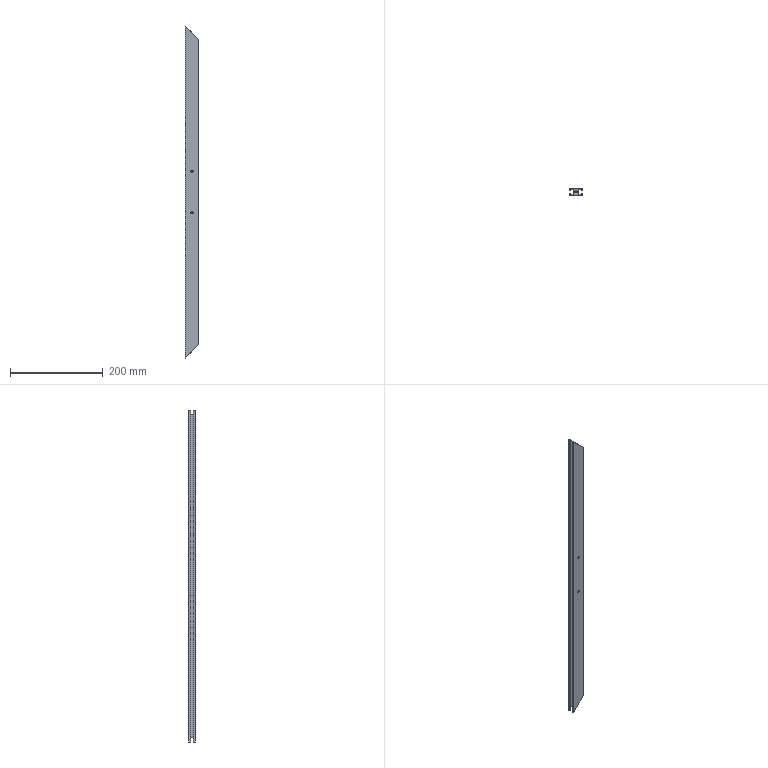Part | SolidWorks | features Extrusion 1, HoleWzd 1, ICE 1 | 1 solid | 37 faces | box 30 x 15 x 717 mm | volume 163444 mm3 | plane 20 | cylinder 17 | commonest cylinder face diameters 5 x14 16.345 x2 16.33 x1
STEP:
#1=CARTESIAN_POINT('',(2375.427,422.907,-45.));
#2=VERTEX_POINT('',#1);
#3=CARTESIAN_POINT('',(2377.927,425.407,-47.5));
#4=VERTEX_POINT('',#3);
#5=CARTESIAN_POINT('',(2375.427,422.907,-45.));
#6=CARTESIAN_POINT('',(2375.427,424.371,-46.464));
#7=CARTESIAN_POINT('',(2376.463,425.407,-47.5));
#8=CARTESIAN_POINT('',(2377.927,425.407,-47.5));
#9=(BOUNDED_CURVE()B_SPLINE_CURVE(3,(#5,#6,#7,#8),.UNSPECIFIED.,.F.,.F.)B_SPLINE_CURVE_WITH_KNOTS((4,4),(4.712,6.283),.UNSPECIFIED.)CURVE()GEOMETRIC_REPRESENTATION_ITEM()RATIONAL_B_SPLINE_CURVE((1.,0.8047,0.8047,1.))REPRESENTATION_ITEM(''));
#10=EDGE_CURVE('',#2,#4,#9,.T.);
#11=ORIENTED_EDGE('',*,*,#10,.T.);
#12=CARTESIAN_POINT('',(2377.927,430.407,-47.5));
#13=VERTEX_POINT('',#12);
#14=CARTESIAN_POINT('',(2377.927,430.407,-47.5));
#15=DIRECTION('',(0.,1.,0.));
#16=VECTOR('',#15,1000.);
#17=LINE('',#14,#16);
#18=EDGE_CURVE('',#4,#13,#17,.T.);
#19=ORIENTED_EDGE('',*,*,#18,.T.);
#20=CARTESIAN_POINT('',(2377.927,430.407,-42.5));
#21=VERTEX_POINT('',#20);
#22=CARTESIAN_POINT('',(2377.927,430.407,-45.));
#23=DIRECTION('',(0.,1.,0.));
#24=DIRECTION('',(0.,0.,1.));
#25=AXIS2_PLACEMENT_3D('',#22,#23,#24);
#26=CIRCLE('',#25,2.5);
#27=EDGE_CURVE('',#13,#21,#26,.T.);
#28=ORIENTED_EDGE('',*,*,#27,.T.);
#29=CARTESIAN_POINT('',(2377.927,425.407,-42.5));
#30=VERTEX_POINT('',#29);
#31=CARTESIAN_POINT('',(2377.927,430.407,-42.5));
#32=DIRECTION('',(0.,1.,0.));
#33=VECTOR('',#32,1000.);
#34=LINE('',#31,#33);
#35=EDGE_CURVE('',#30,#21,#34,.T.);
#36=ORIENTED_EDGE('',*,*,#35,.F.);
#37=CARTESIAN_POINT('',(2377.927,425.407,-42.5));
#38=CARTESIAN_POINT('',(2376.463,425.407,-42.5));
#39=CARTESIAN_POINT('',(2375.427,424.371,-43.536));
#40=CARTESIAN_POINT('',(2375.427,422.907,-45.));
#41=(BOUNDED_CURVE()B_SPLINE_CURVE(3,(#37,#38,#39,#40),.UNSPECIFIED.,.F.,.F.)B_SPLINE_CURVE_WITH_KNOTS((4,4),(3.142,4.712),.UNSPECIFIED.)CURVE()GEOMETRIC_REPRESENTATION_ITEM()RATIONAL_B_SPLINE_CURVE((1.,0.8047,0.8047,1.))REPRESENTATION_ITEM(''));
#42=EDGE_CURVE('',#30,#2,#41,.T.);
#43=ORIENTED_EDGE('',*,*,#42,.T.);
#44=EDGE_LOOP('',(#11,#19,#28,#36,#43));
#45=FACE_OUTER_BOUND('',#44,.T.);
#46=CARTESIAN_POINT('',(2377.927,430.407,-45.));
#47=DIRECTION('',(0.,1.,0.));
#48=DIRECTION('',(0.,0.,1.));
#49=AXIS2_PLACEMENT_3D('',#46,#47,#48);
#50=CYLINDRICAL_SURFACE('',#49,2.5);
#51=ADVANCED_FACE('',(#45),#50,.F.);
#52=CARTESIAN_POINT('',(2377.927,415.407,-47.5));
#53=VERTEX_POINT('',#52);
#54=CARTESIAN_POINT('',(2377.927,415.407,-42.5));
#55=VERTEX_POINT('',#54);
#56=CARTESIAN_POINT('',(2377.927,415.407,-45.));
#57=DIRECTION('',(0.,1.,0.));
#58=DIRECTION('',(0.,0.,1.));
#59=AXIS2_PLACEMENT_3D('',#56,#57,#58);
#60=CIRCLE('',#59,2.5);
#61=EDGE_CURVE('',#53,#55,#60,.T.);
#62=ORIENTED_EDGE('',*,*,#61,.F.);
#63=CARTESIAN_POINT('',(2377.927,420.407,-47.5));
#64=VERTEX_POINT('',#63);
#65=CARTESIAN_POINT('',(2377.927,430.407,-47.5));
#66=DIRECTION('',(0.,1.,0.));
#67=VECTOR('',#66,1000.);
#68=LINE('',#65,#67);
#69=EDGE_CURVE('',#53,#64,#68,.T.);
#70=ORIENTED_EDGE('',*,*,#69,.T.);
#71=CARTESIAN_POINT('',(2377.927,420.407,-47.5));
#72=CARTESIAN_POINT('',(2376.463,420.407,-47.5));
#73=CARTESIAN_POINT('',(2375.427,421.442,-46.464));
#74=CARTESIAN_POINT('',(2375.427,422.907,-45.));
#75=(BOUNDED_CURVE()B_SPLINE_CURVE(3,(#71,#72,#73,#74),.UNSPECIFIED.,.F.,.F.)B_SPLINE_CURVE_WITH_KNOTS((4,4),(0.,1.571),.UNSPECIFIED.)CURVE()GEOMETRIC_REPRESENTATION_ITEM()RATIONAL_B_SPLINE_CURVE((1.,0.8047,0.8047,1.))REPRESENTATION_ITEM(''));
#76=EDGE_CURVE('',#64,#2,#75,.T.);
#77=ORIENTED_EDGE('',*,*,#76,.T.);
#78=CARTESIAN_POINT('',(2377.927,420.407,-42.5));
#79=VERTEX_POINT('',#78);
#80=CARTESIAN_POINT('',(2375.427,422.907,-45.));
#81=CARTESIAN_POINT('',(2375.427,421.442,-43.536));
#82=CARTESIAN_POINT('',(2376.463,420.407,-42.5));
#83=CARTESIAN_POINT('',(2377.927,420.407,-42.5));
#84=(BOUNDED_CURVE()B_SPLINE_CURVE(3,(#80,#81,#82,#83),.UNSPECIFIED.,.F.,.F.)B_SPLINE_CURVE_WITH_KNOTS((4,4),(1.571,3.142),.UNSPECIFIED.)CURVE()GEOMETRIC_REPRESENTATION_ITEM()RATIONAL_B_SPLINE_CURVE((1.,0.8047,0.8047,1.))REPRESENTATION_ITEM(''));
#85=EDGE_CURVE('',#2,#79,#84,.T.);
#86=ORIENTED_EDGE('',*,*,#85,.T.);
#87=CARTESIAN_POINT('',(2377.927,430.407,-42.5));
#88=DIRECTION('',(0.,1.,0.));
#89=VECTOR('',#88,1000.);
#90=LINE('',#87,#89);
#91=EDGE_CURVE('',#55,#79,#90,.T.);
#92=ORIENTED_EDGE('',*,*,#91,.F.);
#93=EDGE_LOOP('',(#62,#70,#77,#86,#92));
#94=FACE_OUTER_BOUND('',#93,.T.);
#95=CARTESIAN_POINT('',(2377.927,430.407,-45.));
#96=DIRECTION('',(0.,1.,0.));
#97=DIRECTION('',(0.,0.,1.));
#98=AXIS2_PLACEMENT_3D('',#95,#96,#97);
#99=CYLINDRICAL_SURFACE('',#98,2.5);
#100=ADVANCED_FACE('',(#94),#99,.F.);
#101=CARTESIAN_POINT('',(2375.427,422.907,45.));
#102=VERTEX_POINT('',#101);
#103=CARTESIAN_POINT('',(2377.927,425.407,42.5));
#104=VERTEX_POINT('',#103);
#105=CARTESIAN_POINT('',(2375.427,422.907,45.));
#106=CARTESIAN_POINT('',(2375.427,424.371,43.536));
#107=CARTESIAN_POINT('',(2376.463,425.407,42.5));
#108=CARTESIAN_POINT('',(2377.927,425.407,42.5));
#109=(BOUNDED_CURVE()B_SPLINE_CURVE(3,(#105,#106,#107,#108),.UNSPECIFIED.,.F.,.F.)B_SPLINE_CURVE_WITH_KNOTS((4,4),(4.712,6.283),.UNSPECIFIED.)CURVE()GEOMETRIC_REPRESENTATION_ITEM()RATIONAL_B_SPLINE_CURVE((1.,0.8047,0.8047,1.))REPRESENTATION_ITEM(''));
#110=EDGE_CURVE('',#102,#104,#109,.T.);
#111=ORIENTED_EDGE('',*,*,#110,.T.);
#112=CARTESIAN_POINT('',(2377.927,430.407,42.5));
#113=VERTEX_POINT('',#112);
#114=CARTESIAN_POINT('',(2377.927,430.407,42.5));
#115=DIRECTION('',(0.,1.,0.));
#116=VECTOR('',#115,1000.);
#117=LINE('',#114,#116);
#118=EDGE_CURVE('',#104,#113,#117,.T.);
#119=ORIENTED_EDGE('',*,*,#118,.T.);
#120=CARTESIAN_POINT('',(2377.927,430.407,47.5));
#121=VERTEX_POINT('',#120);
#122=CARTESIAN_POINT('',(2377.927,430.407,45.));
#123=DIRECTION('',(0.,1.,0.));
#124=DIRECTION('',(0.,0.,1.));
#125=AXIS2_PLACEMENT_3D('',#122,#123,#124);
#126=CIRCLE('',#125,2.5);
#127=EDGE_CURVE('',#113,#121,#126,.T.);
#128=ORIENTED_EDGE('',*,*,#127,.T.);
#129=CARTESIAN_POINT('',(2377.927,425.407,47.5));
#130=VERTEX_POINT('',#129);
#131=CARTESIAN_POINT('',(2377.927,430.407,47.5));
#132=DIRECTION('',(0.,1.,0.));
#133=VECTOR('',#132,1000.);
#134=LINE('',#131,#133);
#135=EDGE_CURVE('',#130,#121,#134,.T.);
#136=ORIENTED_EDGE('',*,*,#135,.F.);
#137=CARTESIAN_POINT('',(2377.927,425.407,47.5));
#138=CARTESIAN_POINT('',(2376.463,425.407,47.5));
#139=CARTESIAN_POINT('',(2375.427,424.371,46.464));
#140=CARTESIAN_POINT('',(2375.427,422.907,45.));
#141=(BOUNDED_CURVE()B_SPLINE_CURVE(3,(#137,#138,#139,#140),.UNSPECIFIED.,.F.,.F.)B_SPLINE_CURVE_WITH_KNOTS((4,4),(3.142,4.712),.UNSPECIFIED.)CURVE()GEOMETRIC_REPRESENTATION_ITEM()RATIONAL_B_SPLINE_CURVE((1.,0.8047,0.8047,1.))REPRESENTATION_ITEM(''));
#142=EDGE_CURVE('',#130,#102,#141,.T.);
#143=ORIENTED_EDGE('',*,*,#142,.T.);
#144=EDGE_LOOP('',(#111,#119,#128,#136,#143));
#145=FACE_OUTER_BOUND('',#144,.T.);
#146=CARTESIAN_POINT('',(2377.927,430.407,45.));
#147=DIRECTION('',(0.,1.,0.));
#148=DIRECTION('',(0.,0.,1.));
#149=AXIS2_PLACEMENT_3D('',#146,#147,#148);
#150=CYLINDRICAL_SURFACE('',#149,2.5);
#151=ADVANCED_FACE('',(#145),#150,.F.);
#152=CARTESIAN_POINT('',(2377.927,415.407,42.5));
#153=VERTEX_POINT('',#152);
#154=CARTESIAN_POINT('',(2377.927,415.407,47.5));
#155=VERTEX_POINT('',#154);
#156=CARTESIAN_POINT('',(2377.927,415.407,45.));
#157=DIRECTION('',(0.,1.,0.));
#158=DIRECTION('',(0.,0.,1.));
#159=AXIS2_PLACEMENT_3D('',#156,#157,#158);
#160=CIRCLE('',#159,2.5);
#161=EDGE_CURVE('',#153,#155,#160,.T.);
#162=ORIENTED_EDGE('',*,*,#161,.F.);
#163=CARTESIAN_POINT('',(2377.927,420.407,42.5));
#164=VERTEX_POINT('',#163);
#165=CARTESIAN_POINT('',(2377.927,430.407,42.5));
#166=DIRECTION('',(0.,1.,0.));
#167=VECTOR('',#166,1000.);
#168=LINE('',#165,#167);
#169=EDGE_CURVE('',#153,#164,#168,.T.);
#170=ORIENTED_EDGE('',*,*,#169,.T.);
#171=CARTESIAN_POINT('',(2377.927,420.407,42.5));
#172=CARTESIAN_POINT('',(2376.463,420.407,42.5));
#173=CARTESIAN_POINT('',(2375.427,421.442,43.536));
#174=CARTESIAN_POINT('',(2375.427,422.907,45.));
#175=(BOUNDED_CURVE()B_SPLINE_CURVE(3,(#171,#172,#173,#174),.UNSPECIFIED.,.F.,.F.)B_SPLINE_CURVE_WITH_KNOTS((4,4),(0.,1.571),.UNSPECIFIED.)CURVE()GEOMETRIC_REPRESENTATION_ITEM()RATIONAL_B_SPLINE_CURVE((1.,0.8047,0.8047,1.))REPRESENTATION_ITEM(''));
#176=EDGE_CURVE('',#164,#102,#175,.T.);
#177=ORIENTED_EDGE('',*,*,#176,.T.);
#178=CARTESIAN_POINT('',(2377.927,420.407,47.5));
#179=VERTEX_POINT('',#178);
#180=CARTESIAN_POINT('',(2375.427,422.907,45.));
#181=CARTESIAN_POINT('',(2375.427,421.442,46.464));
#182=CARTESIAN_POINT('',(2376.463,420.407,47.5));
#183=CARTESIAN_POINT('',(2377.927,420.407,47.5));
#184=(BOUNDED_CURVE()B_SPLINE_CURVE(3,(#180,#181,#182,#183),.UNSPECIFIED.,.F.,.F.)B_SPLINE_CURVE_WITH_KNOTS((4,4),(1.571,3.142),.UNSPECIFIED.)CURVE()GEOMETRIC_REPRESENTATION_ITEM()RATIONAL_B_SPLINE_CURVE((1.,0.8047,0.8047,1.))REPRESENTATION_ITEM(''));
#185=EDGE_CURVE('',#102,#179,#184,.T.);
#186=ORIENTED_EDGE('',*,*,#185,.T.);
#187=CARTESIAN_POINT('',(2377.927,430.407,47.5));
#188=DIRECTION('',(0.,1.,0.));
#189=VECTOR('',#188,1000.);
#190=LINE('',#187,#189);
#191=EDGE_CURVE('',#155,#179,#190,.T.);
#192=ORIENTED_EDGE('',*,*,#191,.F.);
#193=EDGE_LOOP('',(#162,#170,#177,#186,#192));
#194=FACE_OUTER_BOUND('',#193,.T.);
#195=CARTESIAN_POINT('',(2377.927,430.407,45.));
#196=DIRECTION('',(0.,1.,0.));
#197=DIRECTION('',(0.,0.,1.));
#198=AXIS2_PLACEMENT_3D('',#195,#196,#197);
#199=CYLINDRICAL_SURFACE('',#198,2.5);
#200=ADVANCED_FACE('',(#194),#199,.F.);
#201=CARTESIAN_POINT('',(2380.427,422.907,-45.));
#202=VERTEX_POINT('',#201);
#203=CARTESIAN_POINT('',(2380.427,422.907,-45.));
#204=CARTESIAN_POINT('',(2380.427,421.442,-46.464));
#205=CARTESIAN_POINT('',(2379.392,420.407,-47.5));
#206=CARTESIAN_POINT('',(2377.927,420.407,-47.5));
#207=(BOUNDED_CURVE()B_SPLINE_CURVE(3,(#203,#204,#205,#206),.UNSPECIFIED.,.F.,.F.)B_SPLINE_CURVE_WITH_KNOTS((4,4),(4.712,6.283),.UNSPECIFIED.)CURVE()GEOMETRIC_REPRESENTATION_ITEM()RATIONAL_B_SPLINE_CURVE((1.,0.8047,0.8047,1.))REPRESENTATION_ITEM(''));
#208=EDGE_CURVE('',#202,#64,#207,.T.);
#209=ORIENTED_EDGE('',*,*,#208,.F.);
#210=CARTESIAN_POINT('',(2380.427,422.907,-341.));
#211=VERTEX_POINT('',#210);
#212=CARTESIAN_POINT('',(2380.427,422.907,358.5));
#213=DIRECTION('',(0.,0.,-1.));
#214=VECTOR('',#213,1000.);
#215=LINE('',#212,#214);
#216=EDGE_CURVE('',#202,#211,#215,.T.);
#217=ORIENTED_EDGE('',*,*,#216,.T.);
#218=CARTESIAN_POINT('',(2375.427,422.907,-346.));
#219=VERTEX_POINT('',#218);
#220=CARTESIAN_POINT('',(2375.427,422.907,-346.));
#221=CARTESIAN_POINT('',(2375.427,417.907,-346.));
#222=CARTESIAN_POINT('',(2380.427,417.907,-341.));
#223=CARTESIAN_POINT('',(2380.427,422.907,-341.));
#224=(BOUNDED_CURVE()B_SPLINE_CURVE(3,(#220,#221,#222,#223),.UNSPECIFIED.,.F.,.F.)B_SPLINE_CURVE_WITH_KNOTS((4,4),(0.,3.142),.UNSPECIFIED.)CURVE()GEOMETRIC_REPRESENTATION_ITEM()RATIONAL_B_SPLINE_CURVE((1.,0.3333,0.3333,1.))REPRESENTATION_ITEM(''));
#225=EDGE_CURVE('',#219,#211,#224,.T.);
#226=ORIENTED_EDGE('',*,*,#225,.F.);
#227=CARTESIAN_POINT('',(2375.427,422.907,358.5));
#228=DIRECTION('',(0.,0.,-1.));
#229=VECTOR('',#228,1000.);
#230=LINE('',#227,#229);
#231=EDGE_CURVE('',#2,#219,#230,.T.);
#232=ORIENTED_EDGE('',*,*,#231,.F.);
#233=ORIENTED_EDGE('',*,*,#76,.F.);
#234=EDGE_LOOP('',(#209,#217,#226,#232,#233));
#235=FACE_OUTER_BOUND('',#234,.T.);
#236=CARTESIAN_POINT('',(2377.927,422.907,358.5));
#237=DIRECTION('',(0.,0.,-1.));
#238=DIRECTION('',(-1.,0.,0.));
#239=AXIS2_PLACEMENT_3D('',#236,#237,#238);
#240=CYLINDRICAL_SURFACE('',#239,2.5);
#241=ADVANCED_FACE('',(#235),#240,.F.);
#242=CARTESIAN_POINT('',(2382.127,422.907,339.3));
#243=VERTEX_POINT('',#242);
#244=CARTESIAN_POINT('',(2383.995,428.107,337.432));
#245=VERTEX_POINT('',#244);
#246=CARTESIAN_POINT('',(2382.127,422.907,339.3));
#247=CARTESIAN_POINT('',(2382.127,424.824,339.3));
#248=CARTESIAN_POINT('',(2382.775,426.628,338.652));
#249=CARTESIAN_POINT('',(2383.995,428.107,337.432));
#250=(BOUNDED_CURVE()B_SPLINE_CURVE(3,(#246,#247,#248,#249),.UNSPECIFIED.,.F.,.F.)B_SPLINE_CURVE_WITH_KNOTS((4,4),(3.142,3.831),.UNSPECIFIED.)CURVE()GEOMETRIC_REPRESENTATION_ITEM()RATIONAL_B_SPLINE_CURVE((1.,0.9608,0.9608,1.))REPRESENTATION_ITEM(''));
#251=EDGE_CURVE('',#243,#245,#250,.T.);
#252=ORIENTED_EDGE('',*,*,#251,.F.);
#253=CARTESIAN_POINT('',(2382.127,422.907,-339.3));
#254=VERTEX_POINT('',#253);
#255=CARTESIAN_POINT('',(2382.127,422.907,358.5));
#256=DIRECTION('',(0.,0.,-1.));
#257=VECTOR('',#256,1000.);
#258=LINE('',#255,#257);
#259=EDGE_CURVE('',#243,#254,#258,.T.);
#260=ORIENTED_EDGE('',*,*,#259,.T.);
#261=CARTESIAN_POINT('',(2383.995,428.107,-337.432));
#262=VERTEX_POINT('',#261);
#263=CARTESIAN_POINT('',(2383.995,428.107,-337.432));
#264=CARTESIAN_POINT('',(2382.775,426.628,-338.652));
#265=CARTESIAN_POINT('',(2382.127,424.824,-339.3));
#266=CARTESIAN_POINT('',(2382.127,422.907,-339.3));
#267=(BOUNDED_CURVE()B_SPLINE_CURVE(3,(#263,#264,#265,#266),.UNSPECIFIED.,.F.,.T.)B_SPLINE_CURVE_WITH_KNOTS((4,4),(5.594,6.283),.UNSPECIFIED.)CURVE()GEOMETRIC_REPRESENTATION_ITEM()RATIONAL_B_SPLINE_CURVE((1.,0.9608,0.9608,1.))REPRESENTATION_ITEM(''));
#268=EDGE_CURVE('',#262,#254,#267,.T.);
#269=ORIENTED_EDGE('',*,*,#268,.F.);
#270=CARTESIAN_POINT('',(2383.995,428.107,358.5));
#271=DIRECTION('',(0.,0.,-1.));
#272=VECTOR('',#271,1000.);
#273=LINE('',#270,#272);
#274=EDGE_CURVE('',#245,#262,#273,.T.);
#275=ORIENTED_EDGE('',*,*,#274,.F.);
#276=EDGE_LOOP('',(#252,#260,#269,#275));
#277=FACE_OUTER_BOUND('',#276,.T.);
#278=CARTESIAN_POINT('',(2390.3,422.907,358.5));
#279=DIRECTION('',(0.,0.,-1.));
#280=DIRECTION('',(-1.,0.,0.));
#281=AXIS2_PLACEMENT_3D('',#278,#279,#280);
#282=CYLINDRICAL_SURFACE('',#281,8.173);
#283=ADVANCED_FACE('',(#277),#282,.F.);
#284=CARTESIAN_POINT('',(2380.427,422.907,341.));
#285=VERTEX_POINT('',#284);
#286=CARTESIAN_POINT('',(2375.427,422.907,346.));
#287=VERTEX_POINT('',#286);
#288=CARTESIAN_POINT('',(2380.427,422.907,341.));
#289=CARTESIAN_POINT('',(2380.427,417.907,341.));
#290=CARTESIAN_POINT('',(2375.427,417.907,346.));
#291=CARTESIAN_POINT('',(2375.427,422.907,346.));
#292=(BOUNDED_CURVE()B_SPLINE_CURVE(3,(#288,#289,#290,#291),.UNSPECIFIED.,.F.,.F.)B_SPLINE_CURVE_WITH_KNOTS((4,4),(0.,3.142),.UNSPECIFIED.)CURVE()GEOMETRIC_REPRESENTATION_ITEM()RATIONAL_B_SPLINE_CURVE((1.,0.3333,0.3333,1.))REPRESENTATION_ITEM(''));
#293=EDGE_CURVE('',#285,#287,#292,.T.);
#294=ORIENTED_EDGE('',*,*,#293,.F.);
#295=CARTESIAN_POINT('',(2380.427,422.907,45.));
#296=VERTEX_POINT('',#295);
#297=CARTESIAN_POINT('',(2380.427,422.907,358.5));
#298=DIRECTION('',(0.,0.,-1.));
#299=VECTOR('',#298,1000.);
#300=LINE('',#297,#299);
#301=EDGE_CURVE('',#285,#296,#300,.T.);
#302=ORIENTED_EDGE('',*,*,#301,.T.);
#303=CARTESIAN_POINT('',(2377.927,420.407,47.5));
#304=CARTESIAN_POINT('',(2379.392,420.407,47.5));
#305=CARTESIAN_POINT('',(2380.427,421.442,46.464));
#306=CARTESIAN_POINT('',(2380.427,422.907,45.));
#307=(BOUNDED_CURVE()B_SPLINE_CURVE(3,(#303,#304,#305,#306),.UNSPECIFIED.,.F.,.F.)B_SPLINE_CURVE_WITH_KNOTS((4,4),(3.142,4.712),.UNSPECIFIED.)CURVE()GEOMETRIC_REPRESENTATION_ITEM()RATIONAL_B_SPLINE_CURVE((1.,0.8047,0.8047,1.))REPRESENTATION_ITEM(''));
#308=EDGE_CURVE('',#179,#296,#307,.T.);
#309=ORIENTED_EDGE('',*,*,#308,.F.);
#310=ORIENTED_EDGE('',*,*,#185,.F.);
#311=CARTESIAN_POINT('',(2375.427,422.907,358.5));
#312=DIRECTION('',(0.,0.,-1.));
#313=VECTOR('',#312,1000.);
#314=LINE('',#311,#313);
#315=EDGE_CURVE('',#287,#102,#314,.T.);
#316=ORIENTED_EDGE('',*,*,#315,.F.);
#317=EDGE_LOOP('',(#294,#302,#309,#310,#316));
#318=FACE_OUTER_BOUND('',#317,.T.);
#319=CARTESIAN_POINT('',(2377.927,422.907,358.5));
#320=DIRECTION('',(0.,0.,-1.));
#321=DIRECTION('',(-1.,0.,0.));
#322=AXIS2_PLACEMENT_3D('',#319,#320,#321);
#323=CYLINDRICAL_SURFACE('',#322,2.5);
#324=ADVANCED_FACE('',(#318),#323,.F.);
#325=CARTESIAN_POINT('',(2380.427,422.907,45.));
#326=CARTESIAN_POINT('',(2380.427,421.442,43.536));
#327=CARTESIAN_POINT('',(2379.392,420.407,42.5));
#328=CARTESIAN_POINT('',(2377.927,420.407,42.5));
#329=(BOUNDED_CURVE()B_SPLINE_CURVE(3,(#325,#326,#327,#328),.UNSPECIFIED.,.F.,.F.)B_SPLINE_CURVE_WITH_KNOTS((4,4),(4.712,6.283),.UNSPECIFIED.)CURVE()GEOMETRIC_REPRESENTATION_ITEM()RATIONAL_B_SPLINE_CURVE((1.,0.8047,0.8047,1.))REPRESENTATION_ITEM(''));
#330=EDGE_CURVE('',#296,#164,#329,.T.);
#331=ORIENTED_EDGE('',*,*,#330,.F.);
#332=CARTESIAN_POINT('',(2380.427,422.907,358.5));
#333=DIRECTION('',(0.,0.,-1.));
#334=VECTOR('',#333,1000.);
#335=LINE('',#332,#334);
#336=EDGE_CURVE('',#296,#202,#335,.T.);
#337=ORIENTED_EDGE('',*,*,#336,.T.);
#338=CARTESIAN_POINT('',(2377.927,420.407,-42.5));
#339=CARTESIAN_POINT('',(2379.392,420.407,-42.5));
#340=CARTESIAN_POINT('',(2380.427,421.442,-43.536));
#341=CARTESIAN_POINT('',(2380.427,422.907,-45.));
#342=(BOUNDED_CURVE()B_SPLINE_CURVE(3,(#338,#339,#340,#341),.UNSPECIFIED.,.F.,.F.)B_SPLINE_CURVE_WITH_KNOTS((4,4),(3.142,4.712),.UNSPECIFIED.)CURVE()GEOMETRIC_REPRESENTATION_ITEM()RATIONAL_B_SPLINE_CURVE((1.,0.8047,0.8047,1.))REPRESENTATION_ITEM(''));
#343=EDGE_CURVE('',#79,#202,#342,.T.);
#344=ORIENTED_EDGE('',*,*,#343,.F.);
#345=ORIENTED_EDGE('',*,*,#85,.F.);
#346=CARTESIAN_POINT('',(2375.427,422.907,358.5));
#347=DIRECTION('',(0.,0.,-1.));
#348=VECTOR('',#347,1000.);
#349=LINE('',#346,#348);
#350=EDGE_CURVE('',#102,#2,#349,.T.);
#351=ORIENTED_EDGE('',*,*,#350,.F.);
#352=ORIENTED_EDGE('',*,*,#176,.F.);
#353=EDGE_LOOP('',(#331,#337,#344,#345,#351,#352));
#354=FACE_OUTER_BOUND('',#353,.T.);
#355=CARTESIAN_POINT('',(2377.927,422.907,358.5));
#356=DIRECTION('',(0.,0.,-1.));
#357=DIRECTION('',(-1.,0.,0.));
#358=AXIS2_PLACEMENT_3D('',#355,#356,#357);
#359=CYLINDRICAL_SURFACE('',#358,2.5);
#360=ADVANCED_FACE('',(#354),#359,.F.);
#361=ORIENTED_EDGE('',*,*,#336,.F.);
#362=CARTESIAN_POINT('',(2377.927,425.407,42.5));
#363=CARTESIAN_POINT('',(2379.392,425.407,42.5));
#364=CARTESIAN_POINT('',(2380.427,424.371,43.536));
#365=CARTESIAN_POINT('',(2380.427,422.907,45.));
#366=(BOUNDED_CURVE()B_SPLINE_CURVE(3,(#362,#363,#364,#365),.UNSPECIFIED.,.F.,.F.)B_SPLINE_CURVE_WITH_KNOTS((4,4),(0.,1.571),.UNSPECIFIED.)CURVE()GEOMETRIC_REPRESENTATION_ITEM()RATIONAL_B_SPLINE_CURVE((1.,0.8047,0.8047,1.))REPRESENTATION_ITEM(''));
#367=EDGE_CURVE('',#104,#296,#366,.T.);
#368=ORIENTED_EDGE('',*,*,#367,.F.);
#369=ORIENTED_EDGE('',*,*,#110,.F.);
#370=ORIENTED_EDGE('',*,*,#350,.T.);
#371=ORIENTED_EDGE('',*,*,#42,.F.);
#372=CARTESIAN_POINT('',(2380.427,422.907,-45.));
#373=CARTESIAN_POINT('',(2380.427,424.371,-43.536));
#374=CARTESIAN_POINT('',(2379.392,425.407,-42.5));
#375=CARTESIAN_POINT('',(2377.927,425.407,-42.5));
#376=(BOUNDED_CURVE()B_SPLINE_CURVE(3,(#372,#373,#374,#375),.UNSPECIFIED.,.F.,.F.)B_SPLINE_CURVE_WITH_KNOTS((4,4),(1.571,3.142),.UNSPECIFIED.)CURVE()GEOMETRIC_REPRESENTATION_ITEM()RATIONAL_B_SPLINE_CURVE((1.,0.8047,0.8047,1.))REPRESENTATION_ITEM(''));
#377=EDGE_CURVE('',#202,#30,#376,.T.);
#378=ORIENTED_EDGE('',*,*,#377,.F.);
#379=EDGE_LOOP('',(#361,#368,#369,#370,#371,#378));
#380=FACE_OUTER_BOUND('',#379,.T.);
#381=CARTESIAN_POINT('',(2377.927,422.907,358.5));
#382=DIRECTION('',(0.,0.,-1.));
#383=DIRECTION('',(-1.,0.,0.));
#384=AXIS2_PLACEMENT_3D('',#381,#382,#383);
#385=CYLINDRICAL_SURFACE('',#384,2.5);
#386=ADVANCED_FACE('',(#380),#385,.F.);
#387=ORIENTED_EDGE('',*,*,#301,.F.);
#388=CARTESIAN_POINT('',(2375.427,422.907,346.));
#389=CARTESIAN_POINT('',(2375.427,427.907,346.));
#390=CARTESIAN_POINT('',(2380.427,427.907,341.));
#391=CARTESIAN_POINT('',(2380.427,422.907,341.));
#392=(BOUNDED_CURVE()B_SPLINE_CURVE(3,(#388,#389,#390,#391),.UNSPECIFIED.,.F.,.F.)B_SPLINE_CURVE_WITH_KNOTS((4,4),(3.142,6.283),.UNSPECIFIED.)CURVE()GEOMETRIC_REPRESENTATION_ITEM()RATIONAL_B_SPLINE_CURVE((1.,0.3333,0.3333,1.))REPRESENTATION_ITEM(''));
#393=EDGE_CURVE('',#287,#285,#392,.T.);
#394=ORIENTED_EDGE('',*,*,#393,.F.);
#395=ORIENTED_EDGE('',*,*,#315,.T.);
#396=ORIENTED_EDGE('',*,*,#142,.F.);
#397=CARTESIAN_POINT('',(2380.427,422.907,45.));
#398=CARTESIAN_POINT('',(2380.427,424.371,46.464));
#399=CARTESIAN_POINT('',(2379.392,425.407,47.5));
#400=CARTESIAN_POINT('',(2377.927,425.407,47.5));
#401=(BOUNDED_CURVE()B_SPLINE_CURVE(3,(#397,#398,#399,#400),.UNSPECIFIED.,.F.,.F.)B_SPLINE_CURVE_WITH_KNOTS((4,4),(1.571,3.142),.UNSPECIFIED.)CURVE()GEOMETRIC_REPRESENTATION_ITEM()RATIONAL_B_SPLINE_CURVE((1.,0.8047,0.8047,1.))REPRESENTATION_ITEM(''));
#402=EDGE_CURVE('',#296,#130,#401,.T.);
#403=ORIENTED_EDGE('',*,*,#402,.F.);
#404=EDGE_LOOP('',(#387,#394,#395,#396,#403));
#405=FACE_OUTER_BOUND('',#404,.T.);
#406=CARTESIAN_POINT('',(2377.927,422.907,358.5));
#407=DIRECTION('',(0.,0.,-1.));
#408=DIRECTION('',(-1.,0.,0.));
#409=AXIS2_PLACEMENT_3D('',#406,#407,#408);
#410=CYLINDRICAL_SURFACE('',#409,2.5);
#411=ADVANCED_FACE('',(#405),#410,.F.);
#412=CARTESIAN_POINT('',(2362.927,430.407,-358.5));
#413=VERTEX_POINT('',#412);
#414=CARTESIAN_POINT('',(2362.927,426.057,-358.5));
#415=VERTEX_POINT('',#414);
#416=CARTESIAN_POINT('',(2362.927,430.407,-358.5));
#417=DIRECTION('',(0.,-1.,0.));
#418=VECTOR('',#417,1000.);
#419=LINE('',#416,#418);
#420=EDGE_CURVE('',#413,#415,#419,.T.);
#421=ORIENTED_EDGE('',*,*,#420,.T.);
#422=CARTESIAN_POINT('',(2362.927,426.057,358.5));
#423=VERTEX_POINT('',#422);
#424=CARTESIAN_POINT('',(2362.927,426.057,358.5));
#425=DIRECTION('',(0.,0.,-1.));
#426=VECTOR('',#425,1000.);
#427=LINE('',#424,#426);
#428=EDGE_CURVE('',#423,#415,#427,.T.);
#429=ORIENTED_EDGE('',*,*,#428,.F.);
#430=CARTESIAN_POINT('',(2362.927,430.407,358.5));
#431=VERTEX_POINT('',#430);
#432=CARTESIAN_POINT('',(2362.927,430.407,358.5));
#433=DIRECTION('',(0.,-1.,0.));
#434=VECTOR('',#433,1000.);
#435=LINE('',#432,#434);
#436=EDGE_CURVE('',#431,#423,#435,.T.);
#437=ORIENTED_EDGE('',*,*,#436,.F.);
#438=CARTESIAN_POINT('',(2362.927,430.407,358.5));
#439=DIRECTION('',(0.,0.,-1.));
#440=VECTOR('',#439,1000.);
#441=LINE('',#438,#440);
#442=EDGE_CURVE('',#431,#413,#441,.T.);
#443=ORIENTED_EDGE('',*,*,#442,.T.);
#444=EDGE_LOOP('',(#421,#429,#437,#443));
#445=FACE_OUTER_BOUND('',#444,.T.);
#446=CARTESIAN_POINT('',(2362.927,430.407,358.5));
#447=DIRECTION('',(1.,0.,0.));
#448=DIRECTION('',(0.,0.,-1.));
#449=AXIS2_PLACEMENT_3D('',#446,#447,#448);
#450=PLANE('',#449);
#451=ADVANCED_FACE('',(#445),#450,.F.);
#452=CARTESIAN_POINT('',(2365.427,426.057,356.));
#453=VERTEX_POINT('',#452);
#454=CARTESIAN_POINT('',(2364.177,426.057,357.25));
#455=DIRECTION('',(0.7071,0.,-0.7071));
#456=VECTOR('',#455,1000.);
#457=LINE('',#454,#456);
#458=EDGE_CURVE('',#423,#453,#457,.T.);
#459=ORIENTED_EDGE('',*,*,#458,.F.);
#460=ORIENTED_EDGE('',*,*,#428,.T.);
#461=CARTESIAN_POINT('',(2365.427,426.057,-356.));
#462=VERTEX_POINT('',#461);
#463=CARTESIAN_POINT('',(2722.677,426.057,1.25));
#464=DIRECTION('',(-0.7071,0.,-0.7071));
#465=VECTOR('',#464,1000.);
#466=LINE('',#463,#465);
#467=EDGE_CURVE('',#462,#415,#466,.T.);
#468=ORIENTED_EDGE('',*,*,#467,.F.);
#469=CARTESIAN_POINT('',(2365.427,426.057,358.5));
#470=DIRECTION('',(0.,0.,-1.));
#471=VECTOR('',#470,1000.);
#472=LINE('',#469,#471);
#473=EDGE_CURVE('',#453,#462,#472,.T.);
#474=ORIENTED_EDGE('',*,*,#473,.F.);
#475=EDGE_LOOP('',(#459,#460,#468,#474));
#476=FACE_OUTER_BOUND('',#475,.T.);
#477=CARTESIAN_POINT('',(2365.427,426.057,358.5));
#478=DIRECTION('',(0.,-1.,0.));
#479=DIRECTION('',(1.,0.,0.));
#480=AXIS2_PLACEMENT_3D('',#477,#478,#479);
#481=PLANE('',#480);
#482=ADVANCED_FACE('',(#476),#481,.T.);
#483=CARTESIAN_POINT('',(2365.427,428.107,356.));
#484=VERTEX_POINT('',#483);
#485=CARTESIAN_POINT('',(2365.427,428.107,-356.));
#486=VERTEX_POINT('',#485);
#487=CARTESIAN_POINT('',(2365.427,428.107,358.5));
#488=DIRECTION('',(0.,0.,-1.));
#489=VECTOR('',#488,1000.);
#490=LINE('',#487,#489);
#491=EDGE_CURVE('',#484,#486,#490,.T.);
#492=ORIENTED_EDGE('',*,*,#491,.F.);
#493=CARTESIAN_POINT('',(2365.427,426.057,356.));
#494=DIRECTION('',(0.,-1.,0.));
#495=VECTOR('',#494,1000.);
#496=LINE('',#493,#495);
#497=EDGE_CURVE('',#484,#453,#496,.T.);
#498=ORIENTED_EDGE('',*,*,#497,.T.);
#499=ORIENTED_EDGE('',*,*,#473,.T.);
#500=CARTESIAN_POINT('',(2365.427,426.057,-356.));
#501=DIRECTION('',(0.,1.,0.));
#502=VECTOR('',#501,1000.);
#503=LINE('',#500,#502);
#504=EDGE_CURVE('',#462,#486,#503,.T.);
#505=ORIENTED_EDGE('',*,*,#504,.T.);
#506=EDGE_LOOP('',(#492,#498,#499,#505));
#507=FACE_OUTER_BOUND('',#506,.T.);
#508=CARTESIAN_POINT('',(2365.427,426.057,358.5));
#509=DIRECTION('',(-1.,0.,0.));
#510=DIRECTION('',(0.,0.,1.));
#511=AXIS2_PLACEMENT_3D('',#508,#509,#510);
#512=PLANE('',#511);
#513=ADVANCED_FACE('',(#507),#512,.F.);
#514=CARTESIAN_POINT('',(2371.857,428.107,349.57));
#515=VERTEX_POINT('',#514);
#516=CARTESIAN_POINT('',(2371.857,428.107,-349.57));
#517=VERTEX_POINT('',#516);
#518=CARTESIAN_POINT('',(2371.857,428.107,358.5));
#519=DIRECTION('',(0.,0.,-1.));
#520=VECTOR('',#519,1000.);
#521=LINE('',#518,#520);
#522=EDGE_CURVE('',#515,#517,#521,.T.);
#523=ORIENTED_EDGE('',*,*,#522,.F.);
#524=CARTESIAN_POINT('',(2364.177,428.107,357.25));
#525=DIRECTION('',(-0.7071,0.,0.7071));
#526=VECTOR('',#525,1000.);
#527=LINE('',#524,#526);
#528=EDGE_CURVE('',#515,#484,#527,.T.);
#529=ORIENTED_EDGE('',*,*,#528,.T.);
#530=ORIENTED_EDGE('',*,*,#491,.T.);
#531=CARTESIAN_POINT('',(2722.677,428.107,1.25));
#532=DIRECTION('',(0.7071,0.,0.7071));
#533=VECTOR('',#532,1000.);
#534=LINE('',#531,#533);
#535=EDGE_CURVE('',#486,#517,#534,.T.);
#536=ORIENTED_EDGE('',*,*,#535,.T.);
#537=EDGE_LOOP('',(#523,#529,#530,#536));
#538=FACE_OUTER_BOUND('',#537,.T.);
#539=CARTESIAN_POINT('',(2365.427,428.107,358.5));
#540=DIRECTION('',(0.,1.,0.));
#541=DIRECTION('',(0.,0.,1.));
#542=AXIS2_PLACEMENT_3D('',#539,#540,#541);
#543=PLANE('',#542);
#544=ADVANCED_FACE('',(#538),#543,.F.);
#545=CARTESIAN_POINT('',(2371.857,417.707,349.57));
#546=VERTEX_POINT('',#545);
#547=CARTESIAN_POINT('',(2371.857,417.707,-349.57));
#548=VERTEX_POINT('',#547);
#549=CARTESIAN_POINT('',(2371.857,417.707,358.5));
#550=DIRECTION('',(0.,0.,-1.));
#551=VECTOR('',#550,1000.);
#552=LINE('',#549,#551);
#553=EDGE_CURVE('',#546,#548,#552,.T.);
#554=ORIENTED_EDGE('',*,*,#553,.F.);
#555=CARTESIAN_POINT('',(2371.857,417.707,349.57));
#556=CARTESIAN_POINT('',(2374.463,420.861,346.964));
#557=CARTESIAN_POINT('',(2374.463,424.952,346.964));
#558=CARTESIAN_POINT('',(2371.857,428.107,349.57));
#559=(BOUNDED_CURVE()B_SPLINE_CURVE(3,(#555,#556,#557,#558),.UNSPECIFIED.,.F.,.F.)B_SPLINE_CURVE_WITH_KNOTS((4,4),(5.593,6.974),.UNSPECIFIED.)CURVE()GEOMETRIC_REPRESENTATION_ITEM()RATIONAL_B_SPLINE_CURVE((1.,0.8473,0.8473,1.))REPRESENTATION_ITEM(''));
#560=EDGE_CURVE('',#546,#515,#559,.T.);
#561=ORIENTED_EDGE('',*,*,#560,.T.);
#562=ORIENTED_EDGE('',*,*,#522,.T.);
#563=CARTESIAN_POINT('',(2371.857,428.107,-349.57));
#564=CARTESIAN_POINT('',(2374.463,424.952,-346.964));
#565=CARTESIAN_POINT('',(2374.463,420.861,-346.964));
#566=CARTESIAN_POINT('',(2371.857,417.707,-349.57));
#567=(BOUNDED_CURVE()B_SPLINE_CURVE(3,(#563,#564,#565,#566),.UNSPECIFIED.,.F.,.F.)B_SPLINE_CURVE_WITH_KNOTS((4,4),(2.451,3.832),.UNSPECIFIED.)CURVE()GEOMETRIC_REPRESENTATION_ITEM()RATIONAL_B_SPLINE_CURVE((1.,0.8473,0.8473,1.))REPRESENTATION_ITEM(''));
#568=EDGE_CURVE('',#517,#548,#567,.T.);
#569=ORIENTED_EDGE('',*,*,#568,.T.);
#570=EDGE_LOOP('',(#554,#561,#562,#569));
#571=FACE_OUTER_BOUND('',#570,.T.);
#572=CARTESIAN_POINT('',(2365.562,422.907,358.5));
#573=DIRECTION('',(0.,0.,-1.));
#574=DIRECTION('',(-1.,0.,0.));
#575=AXIS2_PLACEMENT_3D('',#572,#573,#574);
#576=CYLINDRICAL_SURFACE('',#575,8.165);
#577=ADVANCED_FACE('',(#571),#576,.F.);
#578=CARTESIAN_POINT('',(2365.427,417.707,356.));
#579=VERTEX_POINT('',#578);
#580=CARTESIAN_POINT('',(2364.177,417.707,357.25));
#581=DIRECTION('',(-0.7071,0.,0.7071));
#582=VECTOR('',#581,1000.);
#583=LINE('',#580,#582);
#584=EDGE_CURVE('',#546,#579,#583,.T.);
#585=ORIENTED_EDGE('',*,*,#584,.F.);
#586=ORIENTED_EDGE('',*,*,#553,.T.);
#587=CARTESIAN_POINT('',(2365.427,417.707,-356.));
#588=VERTEX_POINT('',#587);
#589=CARTESIAN_POINT('',(2722.677,417.707,1.25));
#590=DIRECTION('',(0.7071,0.,0.7071));
#591=VECTOR('',#590,1000.);
#592=LINE('',#589,#591);
#593=EDGE_CURVE('',#588,#548,#592,.T.);
#594=ORIENTED_EDGE('',*,*,#593,.F.);
#595=CARTESIAN_POINT('',(2365.427,417.707,358.5));
#596=DIRECTION('',(0.,0.,-1.));
#597=VECTOR('',#596,1000.);
#598=LINE('',#595,#597);
#599=EDGE_CURVE('',#579,#588,#598,.T.);
#600=ORIENTED_EDGE('',*,*,#599,.F.);
#601=EDGE_LOOP('',(#585,#586,#594,#600));
#602=FACE_OUTER_BOUND('',#601,.T.);
#603=CARTESIAN_POINT('',(2365.427,417.707,358.5));
#604=DIRECTION('',(0.,1.,0.));
#605=DIRECTION('',(0.,0.,1.));
#606=AXIS2_PLACEMENT_3D('',#603,#604,#605);
#607=PLANE('',#606);
#608=ADVANCED_FACE('',(#602),#607,.T.);
#609=CARTESIAN_POINT('',(2365.427,419.757,356.));
#610=VERTEX_POINT('',#609);
#611=CARTESIAN_POINT('',(2365.427,419.757,356.));
#612=DIRECTION('',(0.,1.,0.));
#613=VECTOR('',#612,1000.);
#614=LINE('',#611,#613);
#615=EDGE_CURVE('',#579,#610,#614,.T.);
#616=ORIENTED_EDGE('',*,*,#615,.F.);
#617=ORIENTED_EDGE('',*,*,#599,.T.);
#618=CARTESIAN_POINT('',(2365.427,419.757,-356.));
#619=VERTEX_POINT('',#618);
#620=CARTESIAN_POINT('',(2365.427,419.757,-356.));
#621=DIRECTION('',(0.,-1.,0.));
#622=VECTOR('',#621,1000.);
#623=LINE('',#620,#622);
#624=EDGE_CURVE('',#619,#588,#623,.T.);
#625=ORIENTED_EDGE('',*,*,#624,.F.);
#626=CARTESIAN_POINT('',(2365.427,419.757,358.5));
#627=DIRECTION('',(0.,0.,-1.));
#628=VECTOR('',#627,1000.);
#629=LINE('',#626,#628);
#630=EDGE_CURVE('',#610,#619,#629,.T.);
#631=ORIENTED_EDGE('',*,*,#630,.F.);
#632=EDGE_LOOP('',(#616,#617,#625,#631));
#633=FACE_OUTER_BOUND('',#632,.T.);
#634=CARTESIAN_POINT('',(2365.427,419.757,358.5));
#635=DIRECTION('',(1.,0.,0.));
#636=DIRECTION('',(0.,0.,-1.));
#637=AXIS2_PLACEMENT_3D('',#634,#635,#636);
#638=PLANE('',#637);
#639=ADVANCED_FACE('',(#633),#638,.T.);
#640=CARTESIAN_POINT('',(2362.927,419.757,358.5));
#641=VERTEX_POINT('',#640);
#642=CARTESIAN_POINT('',(2362.927,419.757,-358.5));
#643=VERTEX_POINT('',#642);
#644=CARTESIAN_POINT('',(2362.927,419.757,358.5));
#645=DIRECTION('',(0.,0.,-1.));
#646=VECTOR('',#645,1000.);
#647=LINE('',#644,#646);
#648=EDGE_CURVE('',#641,#643,#647,.T.);
#649=ORIENTED_EDGE('',*,*,#648,.F.);
#650=CARTESIAN_POINT('',(2364.177,419.757,357.25));
#651=DIRECTION('',(0.7071,0.,-0.7071));
#652=VECTOR('',#651,1000.);
#653=LINE('',#650,#652);
#654=EDGE_CURVE('',#641,#610,#653,.T.);
#655=ORIENTED_EDGE('',*,*,#654,.T.);
#656=ORIENTED_EDGE('',*,*,#630,.T.);
#657=CARTESIAN_POINT('',(2722.677,419.757,1.25));
#658=DIRECTION('',(-0.7071,0.,-0.7071));
#659=VECTOR('',#658,1000.);
#660=LINE('',#657,#659);
#661=EDGE_CURVE('',#619,#643,#660,.T.);
#662=ORIENTED_EDGE('',*,*,#661,.T.);
#663=EDGE_LOOP('',(#649,#655,#656,#662));
#664=FACE_OUTER_BOUND('',#663,.T.);
#665=CARTESIAN_POINT('',(2365.427,419.757,358.5));
#666=DIRECTION('',(0.,-1.,0.));
#667=DIRECTION('',(0.,0.,-1.));
#668=AXIS2_PLACEMENT_3D('',#665,#666,#667);
#669=PLANE('',#668);
#670=ADVANCED_FACE('',(#664),#669,.F.);
#671=CARTESIAN_POINT('',(2362.927,415.407,-358.5));
#672=VERTEX_POINT('',#671);
#673=CARTESIAN_POINT('',(2362.927,415.407,-358.5));
#674=DIRECTION('',(0.,1.,0.));
#675=VECTOR('',#674,1000.);
#676=LINE('',#673,#675);
#677=EDGE_CURVE('',#672,#643,#676,.T.);
#678=ORIENTED_EDGE('',*,*,#677,.F.);
#679=CARTESIAN_POINT('',(2362.927,415.407,358.5));
#680=VERTEX_POINT('',#679);
#681=CARTESIAN_POINT('',(2362.927,415.407,358.5));
#682=DIRECTION('',(0.,0.,-1.));
#683=VECTOR('',#682,1000.);
#684=LINE('',#681,#683);
#685=EDGE_CURVE('',#680,#672,#684,.T.);
#686=ORIENTED_EDGE('',*,*,#685,.F.);
#687=CARTESIAN_POINT('',(2362.927,415.407,358.5));
#688=DIRECTION('',(0.,1.,0.));
#689=VECTOR('',#688,1000.);
#690=LINE('',#687,#689);
#691=EDGE_CURVE('',#680,#641,#690,.T.);
#692=ORIENTED_EDGE('',*,*,#691,.T.);
#693=ORIENTED_EDGE('',*,*,#648,.T.);
#694=EDGE_LOOP('',(#678,#686,#692,#693));
#695=FACE_OUTER_BOUND('',#694,.T.);
#696=CARTESIAN_POINT('',(2362.927,415.407,358.5));
#697=DIRECTION('',(-1.,0.,0.));
#698=DIRECTION('',(0.,0.,1.));
#699=AXIS2_PLACEMENT_3D('',#696,#697,#698);
#700=PLANE('',#699);
#701=ADVANCED_FACE('',(#695),#700,.T.);
#702=CARTESIAN_POINT('',(2377.927,415.407,-45.));
#703=DIRECTION('',(0.,1.,0.));
#704=DIRECTION('',(0.,0.,1.));
#705=AXIS2_PLACEMENT_3D('',#702,#703,#704);
#706=CIRCLE('',#705,2.5);
#707=EDGE_CURVE('',#55,#53,#706,.T.);
#708=ORIENTED_EDGE('',*,*,#707,.T.);
#709=ORIENTED_EDGE('',*,*,#61,.T.);
#710=EDGE_LOOP('',(#708,#709));
#711=FACE_BOUND('',#710,.T.);
#712=CARTESIAN_POINT('',(2377.927,415.407,45.));
#713=DIRECTION('',(0.,1.,0.));
#714=DIRECTION('',(0.,0.,1.));
#715=AXIS2_PLACEMENT_3D('',#712,#713,#714);
#716=CIRCLE('',#715,2.5);
#717=EDGE_CURVE('',#155,#153,#716,.T.);
#718=ORIENTED_EDGE('',*,*,#717,.T.);
#719=ORIENTED_EDGE('',*,*,#161,.T.);
#720=EDGE_LOOP('',(#718,#719));
#721=FACE_BOUND('',#720,.T.);
#722=CARTESIAN_POINT('',(2392.927,415.407,328.5));
#723=VERTEX_POINT('',#722);
#724=CARTESIAN_POINT('',(2392.927,415.407,-328.5));
#725=VERTEX_POINT('',#724);
#726=CARTESIAN_POINT('',(2392.927,415.407,358.5));
#727=DIRECTION('',(0.,0.,-1.));
#728=VECTOR('',#727,1000.);
#729=LINE('',#726,#728);
#730=EDGE_CURVE('',#723,#725,#729,.T.);
#731=ORIENTED_EDGE('',*,*,#730,.F.);
#732=CARTESIAN_POINT('',(2362.927,415.407,358.5));
#733=DIRECTION('',(-0.7071,0.,0.7071));
#734=VECTOR('',#733,1000.);
#735=LINE('',#732,#734);
#736=EDGE_CURVE('',#723,#680,#735,.T.);
#737=ORIENTED_EDGE('',*,*,#736,.T.);
#738=ORIENTED_EDGE('',*,*,#685,.T.);
#739=CARTESIAN_POINT('',(2362.927,415.407,-358.5));
#740=DIRECTION('',(0.7071,0.,0.7071));
#741=VECTOR('',#740,1000.);
#742=LINE('',#739,#741);
#743=EDGE_CURVE('',#672,#725,#742,.T.);
#744=ORIENTED_EDGE('',*,*,#743,.T.);
#745=EDGE_LOOP('',(#731,#737,#738,#744));
#746=FACE_OUTER_BOUND('',#745,.T.);
#747=CARTESIAN_POINT('',(2362.927,415.407,358.5));
#748=DIRECTION('',(0.,1.,0.));
#749=DIRECTION('',(0.,0.,1.));
#750=AXIS2_PLACEMENT_3D('',#747,#748,#749);
#751=PLANE('',#750);
#752=ADVANCED_FACE('',(#711,#721,#746),#751,.F.);
#753=CARTESIAN_POINT('',(2392.927,419.757,328.5));
#754=VERTEX_POINT('',#753);
#755=CARTESIAN_POINT('',(2392.927,419.757,-328.5));
#756=VERTEX_POINT('',#755);
#757=CARTESIAN_POINT('',(2392.927,419.757,358.5));
#758=DIRECTION('',(0.,0.,-1.));
#759=VECTOR('',#758,1000.);
#760=LINE('',#757,#759);
#761=EDGE_CURVE('',#754,#756,#760,.T.);
#762=ORIENTED_EDGE('',*,*,#761,.F.);
#763=CARTESIAN_POINT('',(2392.927,415.407,328.5));
#764=DIRECTION('',(0.,1.,0.));
#765=VECTOR('',#764,1000.);
#766=LINE('',#763,#765);
#767=EDGE_CURVE('',#723,#754,#766,.T.);
#768=ORIENTED_EDGE('',*,*,#767,.F.);
#769=ORIENTED_EDGE('',*,*,#730,.T.);
#770=CARTESIAN_POINT('',(2392.927,415.407,-328.5));
#771=DIRECTION('',(0.,1.,0.));
#772=VECTOR('',#771,1000.);
#773=LINE('',#770,#772);
#774=EDGE_CURVE('',#725,#756,#773,.T.);
#775=ORIENTED_EDGE('',*,*,#774,.T.);
#776=EDGE_LOOP('',(#762,#768,#769,#775));
#777=FACE_OUTER_BOUND('',#776,.T.);
#778=CARTESIAN_POINT('',(2392.927,415.407,358.5));
#779=DIRECTION('',(-1.,0.,0.));
#780=DIRECTION('',(0.,0.,1.));
#781=AXIS2_PLACEMENT_3D('',#778,#779,#780);
#782=PLANE('',#781);
#783=ADVANCED_FACE('',(#777),#782,.F.);
#784=CARTESIAN_POINT('',(2390.427,419.757,331.));
#785=VERTEX_POINT('',#784);
#786=CARTESIAN_POINT('',(2376.677,419.757,344.75));
#787=DIRECTION('',(-0.7071,0.,0.7071));
#788=VECTOR('',#787,1000.);
#789=LINE('',#786,#788);
#790=EDGE_CURVE('',#754,#785,#789,.T.);
#791=ORIENTED_EDGE('',*,*,#790,.F.);
#792=ORIENTED_EDGE('',*,*,#761,.T.);
#793=CARTESIAN_POINT('',(2390.427,419.757,-331.));
#794=VERTEX_POINT('',#793);
#795=CARTESIAN_POINT('',(2735.177,419.757,13.75));
#796=DIRECTION('',(0.7071,0.,0.7071));
#797=VECTOR('',#796,1000.);
#798=LINE('',#795,#797);
#799=EDGE_CURVE('',#794,#756,#798,.T.);
#800=ORIENTED_EDGE('',*,*,#799,.F.);
#801=CARTESIAN_POINT('',(2390.427,419.757,358.5));
#802=DIRECTION('',(0.,0.,-1.));
#803=VECTOR('',#802,1000.);
#804=LINE('',#801,#803);
#805=EDGE_CURVE('',#785,#794,#804,.T.);
#806=ORIENTED_EDGE('',*,*,#805,.F.);
#807=EDGE_LOOP('',(#791,#792,#800,#806));
#808=FACE_OUTER_BOUND('',#807,.T.);
#809=CARTESIAN_POINT('',(2390.427,419.757,358.5));
#810=DIRECTION('',(0.,1.,0.));
#811=DIRECTION('',(0.,0.,1.));
#812=AXIS2_PLACEMENT_3D('',#809,#810,#811);
#813=PLANE('',#812);
#814=ADVANCED_FACE('',(#808),#813,.T.);
#815=CARTESIAN_POINT('',(2390.427,417.707,331.));
#816=VERTEX_POINT('',#815);
#817=CARTESIAN_POINT('',(2390.427,417.707,-331.));
#818=VERTEX_POINT('',#817);
#819=CARTESIAN_POINT('',(2390.427,417.707,358.5));
#820=DIRECTION('',(0.,0.,-1.));
#821=VECTOR('',#820,1000.);
#822=LINE('',#819,#821);
#823=EDGE_CURVE('',#816,#818,#822,.T.);
#824=ORIENTED_EDGE('',*,*,#823,.F.);
#825=CARTESIAN_POINT('',(2390.427,419.757,331.));
#826=DIRECTION('',(0.,1.,0.));
#827=VECTOR('',#826,1000.);
#828=LINE('',#825,#827);
#829=EDGE_CURVE('',#816,#785,#828,.T.);
#830=ORIENTED_EDGE('',*,*,#829,.T.);
#831=ORIENTED_EDGE('',*,*,#805,.T.);
#832=CARTESIAN_POINT('',(2390.427,419.757,-331.));
#833=DIRECTION('',(0.,-1.,0.));
#834=VECTOR('',#833,1000.);
#835=LINE('',#832,#834);
#836=EDGE_CURVE('',#794,#818,#835,.T.);
#837=ORIENTED_EDGE('',*,*,#836,.T.);
#838=EDGE_LOOP('',(#824,#830,#831,#837));
#839=FACE_OUTER_BOUND('',#838,.T.);
#840=CARTESIAN_POINT('',(2390.427,419.757,358.5));
#841=DIRECTION('',(1.,0.,0.));
#842=DIRECTION('',(0.,0.,-1.));
#843=AXIS2_PLACEMENT_3D('',#840,#841,#842);
#844=PLANE('',#843);
#845=ADVANCED_FACE('',(#839),#844,.F.);
#846=CARTESIAN_POINT('',(2383.995,417.707,337.432));
#847=VERTEX_POINT('',#846);
#848=CARTESIAN_POINT('',(2373.461,417.707,347.966));
#849=DIRECTION('',(-0.7071,0.,0.7071));
#850=VECTOR('',#849,1000.);
#851=LINE('',#848,#850);
#852=EDGE_CURVE('',#816,#847,#851,.T.);
#853=ORIENTED_EDGE('',*,*,#852,.F.);
#854=ORIENTED_EDGE('',*,*,#823,.T.);
#855=CARTESIAN_POINT('',(2383.995,417.707,-337.432));
#856=VERTEX_POINT('',#855);
#857=CARTESIAN_POINT('',(2731.961,417.707,10.534));
#858=DIRECTION('',(0.7071,0.,0.7071));
#859=VECTOR('',#858,1000.);
#860=LINE('',#857,#859);
#861=EDGE_CURVE('',#856,#818,#860,.T.);
#862=ORIENTED_EDGE('',*,*,#861,.F.);
#863=CARTESIAN_POINT('',(2383.995,417.707,358.5));
#864=DIRECTION('',(0.,0.,-1.));
#865=VECTOR('',#864,1000.);
#866=LINE('',#863,#865);
#867=EDGE_CURVE('',#847,#856,#866,.T.);
#868=ORIENTED_EDGE('',*,*,#867,.F.);
#869=EDGE_LOOP('',(#853,#854,#862,#868));
#870=FACE_OUTER_BOUND('',#869,.T.);
#871=CARTESIAN_POINT('',(2383.995,417.707,358.5));
#872=DIRECTION('',(0.,1.,0.));
#873=DIRECTION('',(-1.,0.,0.));
#874=AXIS2_PLACEMENT_3D('',#871,#872,#873);
#875=PLANE('',#874);
#876=ADVANCED_FACE('',(#870),#875,.T.);
#877=ORIENTED_EDGE('',*,*,#259,.F.);
#878=CARTESIAN_POINT('',(2383.995,417.707,337.432));
#879=CARTESIAN_POINT('',(2382.775,419.186,338.652));
#880=CARTESIAN_POINT('',(2382.127,420.99,339.3));
#881=CARTESIAN_POINT('',(2382.127,422.907,339.3));
#882=(BOUNDED_CURVE()B_SPLINE_CURVE(3,(#878,#879,#880,#881),.UNSPECIFIED.,.F.,.F.)B_SPLINE_CURVE_WITH_KNOTS((4,4),(2.452,3.142),.UNSPECIFIED.)CURVE()GEOMETRIC_REPRESENTATION_ITEM()RATIONAL_B_SPLINE_CURVE((1.,0.9608,0.9608,1.))REPRESENTATION_ITEM(''));
#883=EDGE_CURVE('',#847,#243,#882,.T.);
#884=ORIENTED_EDGE('',*,*,#883,.F.);
#885=ORIENTED_EDGE('',*,*,#867,.T.);
#886=CARTESIAN_POINT('',(2382.127,422.907,-339.3));
#887=CARTESIAN_POINT('',(2382.127,420.99,-339.3));
#888=CARTESIAN_POINT('',(2382.775,419.186,-338.652));
#889=CARTESIAN_POINT('',(2383.995,417.707,-337.432));
#890=(BOUNDED_CURVE()B_SPLINE_CURVE(3,(#886,#887,#888,#889),.UNSPECIFIED.,.F.,.F.)B_SPLINE_CURVE_WITH_KNOTS((4,4),(0.,0.6897),.UNSPECIFIED.)CURVE()GEOMETRIC_REPRESENTATION_ITEM()RATIONAL_B_SPLINE_CURVE((1.,0.9608,0.9608,1.))REPRESENTATION_ITEM(''));
#891=EDGE_CURVE('',#254,#856,#890,.T.);
#892=ORIENTED_EDGE('',*,*,#891,.F.);
#893=EDGE_LOOP('',(#877,#884,#885,#892));
#894=FACE_OUTER_BOUND('',#893,.T.);
#895=CARTESIAN_POINT('',(2390.3,422.907,358.5));
#896=DIRECTION('',(0.,0.,-1.));
#897=DIRECTION('',(-1.,0.,0.));
#898=AXIS2_PLACEMENT_3D('',#895,#896,#897);
#899=CYLINDRICAL_SURFACE('',#898,8.173);
#900=ADVANCED_FACE('',(#894),#899,.F.);
#901=CARTESIAN_POINT('',(2390.427,428.107,331.));
#902=VERTEX_POINT('',#901);
#903=CARTESIAN_POINT('',(2390.427,428.107,-331.));
#904=VERTEX_POINT('',#903);
#905=CARTESIAN_POINT('',(2390.427,428.107,358.5));
#906=DIRECTION('',(0.,0.,-1.));
#907=VECTOR('',#906,1000.);
#908=LINE('',#905,#907);
#909=EDGE_CURVE('',#902,#904,#908,.T.);
#910=ORIENTED_EDGE('',*,*,#909,.F.);
#911=CARTESIAN_POINT('',(2373.461,428.107,347.966));
#912=DIRECTION('',(-0.7071,0.,0.7071));
#913=VECTOR('',#912,1000.);
#914=LINE('',#911,#913);
#915=EDGE_CURVE('',#902,#245,#914,.T.);
#916=ORIENTED_EDGE('',*,*,#915,.T.);
#917=ORIENTED_EDGE('',*,*,#274,.T.);
#918=CARTESIAN_POINT('',(2731.961,428.107,10.534));
#919=DIRECTION('',(0.7071,0.,0.7071));
#920=VECTOR('',#919,1000.);
#921=LINE('',#918,#920);
#922=EDGE_CURVE('',#262,#904,#921,.T.);
#923=ORIENTED_EDGE('',*,*,#922,.T.);
#924=EDGE_LOOP('',(#910,#916,#917,#923));
#925=FACE_OUTER_BOUND('',#924,.T.);
#926=CARTESIAN_POINT('',(2383.995,428.107,358.5));
#927=DIRECTION('',(0.,1.,0.));
#928=DIRECTION('',(-1.,0.,0.));
#929=AXIS2_PLACEMENT_3D('',#926,#927,#928);
#930=PLANE('',#929);
#931=ADVANCED_FACE('',(#925),#930,.F.);
#932=CARTESIAN_POINT('',(2390.427,426.057,331.));
#933=VERTEX_POINT('',#932);
#934=CARTESIAN_POINT('',(2390.427,426.057,331.));
#935=DIRECTION('',(0.,-1.,0.));
#936=VECTOR('',#935,1000.);
#937=LINE('',#934,#936);
#938=EDGE_CURVE('',#902,#933,#937,.T.);
#939=ORIENTED_EDGE('',*,*,#938,.F.);
#940=ORIENTED_EDGE('',*,*,#909,.T.);
#941=CARTESIAN_POINT('',(2390.427,426.057,-331.));
#942=VERTEX_POINT('',#941);
#943=CARTESIAN_POINT('',(2390.427,426.057,-331.));
#944=DIRECTION('',(0.,1.,0.));
#945=VECTOR('',#944,1000.);
#946=LINE('',#943,#945);
#947=EDGE_CURVE('',#942,#904,#946,.T.);
#948=ORIENTED_EDGE('',*,*,#947,.F.);
#949=CARTESIAN_POINT('',(2390.427,426.057,358.5));
#950=DIRECTION('',(0.,0.,-1.));
#951=VECTOR('',#950,1000.);
#952=LINE('',#949,#951);
#953=EDGE_CURVE('',#933,#942,#952,.T.);
#954=ORIENTED_EDGE('',*,*,#953,.F.);
#955=EDGE_LOOP('',(#939,#940,#948,#954));
#956=FACE_OUTER_BOUND('',#955,.T.);
#957=CARTESIAN_POINT('',(2390.427,426.057,358.5));
#958=DIRECTION('',(-1.,0.,0.));
#959=DIRECTION('',(0.,0.,1.));
#960=AXIS2_PLACEMENT_3D('',#957,#958,#959);
#961=PLANE('',#960);
#962=ADVANCED_FACE('',(#956),#961,.T.);
#963=CARTESIAN_POINT('',(2392.927,426.057,328.5));
#964=VERTEX_POINT('',#963);
#965=CARTESIAN_POINT('',(2392.927,426.057,-328.5));
#966=VERTEX_POINT('',#965);
#967=CARTESIAN_POINT('',(2392.927,426.057,358.5));
#968=DIRECTION('',(0.,0.,-1.));
#969=VECTOR('',#968,1000.);
#970=LINE('',#967,#969);
#971=EDGE_CURVE('',#964,#966,#970,.T.);
#972=ORIENTED_EDGE('',*,*,#971,.F.);
#973=CARTESIAN_POINT('',(2376.677,426.057,344.75));
#974=DIRECTION('',(-0.7071,0.,0.7071));
#975=VECTOR('',#974,1000.);
#976=LINE('',#973,#975);
#977=EDGE_CURVE('',#964,#933,#976,.T.);
#978=ORIENTED_EDGE('',*,*,#977,.T.);
#979=ORIENTED_EDGE('',*,*,#953,.T.);
#980=CARTESIAN_POINT('',(2735.177,426.057,13.75));
#981=DIRECTION('',(0.7071,0.,0.7071));
#982=VECTOR('',#981,1000.);
#983=LINE('',#980,#982);
#984=EDGE_CURVE('',#942,#966,#983,.T.);
#985=ORIENTED_EDGE('',*,*,#984,.T.);
#986=EDGE_LOOP('',(#972,#978,#979,#985));
#987=FACE_OUTER_BOUND('',#986,.T.);
#988=CARTESIAN_POINT('',(2390.427,426.057,358.5));
#989=DIRECTION('',(0.,1.,0.));
#990=DIRECTION('',(0.,0.,1.));
#991=AXIS2_PLACEMENT_3D('',#988,#989,#990);
#992=PLANE('',#991);
#993=ADVANCED_FACE('',(#987),#992,.F.);
#994=CARTESIAN_POINT('',(2392.927,430.407,328.5));
#995=VERTEX_POINT('',#994);
#996=CARTESIAN_POINT('',(2392.927,415.407,328.5));
#997=DIRECTION('',(0.,1.,0.));
#998=VECTOR('',#997,1000.);
#999=LINE('',#996,#998);
#1000=EDGE_CURVE('',#964,#995,#999,.T.);
#1001=ORIENTED_EDGE('',*,*,#1000,.F.);
#1002=ORIENTED_EDGE('',*,*,#971,.T.);
#1003=CARTESIAN_POINT('',(2392.927,430.407,-328.5));
#1004=VERTEX_POINT('',#1003);
#1005=CARTESIAN_POINT('',(2392.927,415.407,-328.5));
#1006=DIRECTION('',(0.,1.,0.));
#1007=VECTOR('',#1006,1000.);
#1008=LINE('',#1005,#1007);
#1009=EDGE_CURVE('',#966,#1004,#1008,.T.);
#1010=ORIENTED_EDGE('',*,*,#1009,.T.);
#1011=CARTESIAN_POINT('',(2392.927,430.407,358.5));
#1012=DIRECTION('',(0.,0.,-1.));
#1013=VECTOR('',#1012,1000.);
#1014=LINE('',#1011,#1013);
#1015=EDGE_CURVE('',#995,#1004,#1014,.T.);
#1016=ORIENTED_EDGE('',*,*,#1015,.F.);
#1017=EDGE_LOOP('',(#1001,#1002,#1010,#1016));
#1018=FACE_OUTER_BOUND('',#1017,.T.);
#1019=CARTESIAN_POINT('',(2392.927,430.407,358.5));
#1020=DIRECTION('',(1.,0.,0.));
#1021=DIRECTION('',(0.,0.,-1.));
#1022=AXIS2_PLACEMENT_3D('',#1019,#1020,#1021);
#1023=PLANE('',#1022);
#1024=ADVANCED_FACE('',(#1018),#1023,.T.);
#1025=CARTESIAN_POINT('',(2377.927,430.407,-45.));
#1026=DIRECTION('',(0.,1.,0.));
#1027=DIRECTION('',(0.,0.,1.));
#1028=AXIS2_PLACEMENT_3D('',#1025,#1026,#1027);
#1029=CIRCLE('',#1028,2.5);
#1030=EDGE_CURVE('',#21,#13,#1029,.T.);
#1031=ORIENTED_EDGE('',*,*,#1030,.F.);
#1032=ORIENTED_EDGE('',*,*,#27,.F.);
#1033=EDGE_LOOP('',(#1031,#1032));
#1034=FACE_BOUND('',#1033,.T.);
#1035=CARTESIAN_POINT('',(2377.927,430.407,45.));
#1036=DIRECTION('',(0.,1.,0.));
#1037=DIRECTION('',(0.,0.,1.));
#1038=AXIS2_PLACEMENT_3D('',#1035,#1036,#1037);
#1039=CIRCLE('',#1038,2.5);
#1040=EDGE_CURVE('',#121,#113,#1039,.T.);
#1041=ORIENTED_EDGE('',*,*,#1040,.F.);
#1042=ORIENTED_EDGE('',*,*,#127,.F.);
#1043=EDGE_LOOP('',(#1041,#1042));
#1044=FACE_BOUND('',#1043,.T.);
#1045=CARTESIAN_POINT('',(2362.927,430.407,358.5));
#1046=DIRECTION('',(-0.7071,0.,0.7071));
#1047=VECTOR('',#1046,1000.);
#1048=LINE('',#1045,#1047);
#1049=EDGE_CURVE('',#995,#431,#1048,.T.);
#1050=ORIENTED_EDGE('',*,*,#1049,.F.);
#1051=ORIENTED_EDGE('',*,*,#1015,.T.);
#1052=CARTESIAN_POINT('',(2362.927,430.407,-358.5));
#1053=DIRECTION('',(0.7071,0.,0.7071));
#1054=VECTOR('',#1053,1000.);
#1055=LINE('',#1052,#1054);
#1056=EDGE_CURVE('',#413,#1004,#1055,.T.);
#1057=ORIENTED_EDGE('',*,*,#1056,.F.);
#1058=ORIENTED_EDGE('',*,*,#442,.F.);
#1059=EDGE_LOOP('',(#1050,#1051,#1057,#1058));
#1060=FACE_OUTER_BOUND('',#1059,.T.);
#1061=CARTESIAN_POINT('',(2362.927,430.407,358.5));
#1062=DIRECTION('',(0.,1.,0.));
#1063=DIRECTION('',(0.,0.,1.));
#1064=AXIS2_PLACEMENT_3D('',#1061,#1062,#1063);
#1065=PLANE('',#1064);
#1066=ADVANCED_FACE('',(#1034,#1044,#1060),#1065,.T.);
#1067=ORIENTED_EDGE('',*,*,#216,.F.);
#1068=CARTESIAN_POINT('',(2377.927,425.407,-47.5));
#1069=CARTESIAN_POINT('',(2379.392,425.407,-47.5));
#1070=CARTESIAN_POINT('',(2380.427,424.371,-46.464));
#1071=CARTESIAN_POINT('',(2380.427,422.907,-45.));
#1072=(BOUNDED_CURVE()B_SPLINE_CURVE(3,(#1068,#1069,#1070,#1071),.UNSPECIFIED.,.F.,.F.)B_SPLINE_CURVE_WITH_KNOTS((4,4),(0.,1.571),.UNSPECIFIED.)CURVE()GEOMETRIC_REPRESENTATION_ITEM()RATIONAL_B_SPLINE_CURVE((1.,0.8047,0.8047,1.))REPRESENTATION_ITEM(''));
#1073=EDGE_CURVE('',#4,#202,#1072,.T.);
#1074=ORIENTED_EDGE('',*,*,#1073,.F.);
#1075=ORIENTED_EDGE('',*,*,#10,.F.);
#1076=ORIENTED_EDGE('',*,*,#231,.T.);
#1077=CARTESIAN_POINT('',(2380.427,422.907,-341.));
#1078=CARTESIAN_POINT('',(2380.427,427.907,-341.));
#1079=CARTESIAN_POINT('',(2375.427,427.907,-346.));
#1080=CARTESIAN_POINT('',(2375.427,422.907,-346.));
#1081=(BOUNDED_CURVE()B_SPLINE_CURVE(3,(#1077,#1078,#1079,#1080),.UNSPECIFIED.,.F.,.F.)B_SPLINE_CURVE_WITH_KNOTS((4,4),(3.142,6.283),.UNSPECIFIED.)CURVE()GEOMETRIC_REPRESENTATION_ITEM()RATIONAL_B_SPLINE_CURVE((1.,0.3333,0.3333,1.))REPRESENTATION_ITEM(''));
#1082=EDGE_CURVE('',#211,#219,#1081,.T.);
#1083=ORIENTED_EDGE('',*,*,#1082,.F.);
#1084=EDGE_LOOP('',(#1067,#1074,#1075,#1076,#1083));
#1085=FACE_OUTER_BOUND('',#1084,.T.);
#1086=CARTESIAN_POINT('',(2377.927,422.907,358.5));
#1087=DIRECTION('',(0.,0.,-1.));
#1088=DIRECTION('',(-1.,0.,0.));
#1089=AXIS2_PLACEMENT_3D('',#1086,#1087,#1088);
#1090=CYLINDRICAL_SURFACE('',#1089,2.5);
#1091=ADVANCED_FACE('',(#1085),#1090,.F.);
#1092=ORIENTED_EDGE('',*,*,#467,.T.);
#1093=ORIENTED_EDGE('',*,*,#420,.F.);
#1094=ORIENTED_EDGE('',*,*,#1056,.T.);
#1095=ORIENTED_EDGE('',*,*,#1009,.F.);
#1096=ORIENTED_EDGE('',*,*,#984,.F.);
#1097=ORIENTED_EDGE('',*,*,#947,.T.);
#1098=ORIENTED_EDGE('',*,*,#922,.F.);
#1099=ORIENTED_EDGE('',*,*,#268,.T.);
#1100=ORIENTED_EDGE('',*,*,#891,.T.);
#1101=ORIENTED_EDGE('',*,*,#861,.T.);
#1102=ORIENTED_EDGE('',*,*,#836,.F.);
#1103=ORIENTED_EDGE('',*,*,#799,.T.);
#1104=ORIENTED_EDGE('',*,*,#774,.F.);
#1105=ORIENTED_EDGE('',*,*,#743,.F.);
#1106=ORIENTED_EDGE('',*,*,#677,.T.);
#1107=ORIENTED_EDGE('',*,*,#661,.F.);
#1108=ORIENTED_EDGE('',*,*,#624,.T.);
#1109=ORIENTED_EDGE('',*,*,#593,.T.);
#1110=ORIENTED_EDGE('',*,*,#568,.F.);
#1111=ORIENTED_EDGE('',*,*,#535,.F.);
#1112=ORIENTED_EDGE('',*,*,#504,.F.);
#1113=EDGE_LOOP('',(#1092,#1093,#1094,#1095,#1096,#1097,#1098,#1099,#1100,#1101,#1102,#1103,#1104,#1105,#1106,#1107,#1108,#1109,#1110,#1111,#1112));
#1114=FACE_OUTER_BOUND('',#1113,.T.);
#1115=ORIENTED_EDGE('',*,*,#225,.T.);
#1116=ORIENTED_EDGE('',*,*,#1082,.T.);
#1117=EDGE_LOOP('',(#1115,#1116));
#1118=FACE_BOUND('',#1117,.T.);
#1119=CARTESIAN_POINT('',(2362.927,415.407,-358.5));
#1120=DIRECTION('',(-0.7071,0.,0.7071));
#1121=DIRECTION('',(0.7071,0.,0.7071));
#1122=AXIS2_PLACEMENT_3D('',#1119,#1120,#1121);
#1123=PLANE('',#1122);
#1124=ADVANCED_FACE('',(#1114,#1118),#1123,.F.);
#1125=ORIENTED_EDGE('',*,*,#458,.T.);
#1126=ORIENTED_EDGE('',*,*,#497,.F.);
#1127=ORIENTED_EDGE('',*,*,#528,.F.);
#1128=ORIENTED_EDGE('',*,*,#560,.F.);
#1129=ORIENTED_EDGE('',*,*,#584,.T.);
#1130=ORIENTED_EDGE('',*,*,#615,.T.);
#1131=ORIENTED_EDGE('',*,*,#654,.F.);
#1132=ORIENTED_EDGE('',*,*,#691,.F.);
#1133=ORIENTED_EDGE('',*,*,#736,.F.);
#1134=ORIENTED_EDGE('',*,*,#767,.T.);
#1135=ORIENTED_EDGE('',*,*,#790,.T.);
#1136=ORIENTED_EDGE('',*,*,#829,.F.);
#1137=ORIENTED_EDGE('',*,*,#852,.T.);
#1138=ORIENTED_EDGE('',*,*,#883,.T.);
#1139=ORIENTED_EDGE('',*,*,#251,.T.);
#1140=ORIENTED_EDGE('',*,*,#915,.F.);
#1141=ORIENTED_EDGE('',*,*,#938,.T.);
#1142=ORIENTED_EDGE('',*,*,#977,.F.);
#1143=ORIENTED_EDGE('',*,*,#1000,.T.);
#1144=ORIENTED_EDGE('',*,*,#1049,.T.);
#1145=ORIENTED_EDGE('',*,*,#436,.T.);
#1146=EDGE_LOOP('',(#1125,#1126,#1127,#1128,#1129,#1130,#1131,#1132,#1133,#1134,#1135,#1136,#1137,#1138,#1139,#1140,#1141,#1142,#1143,#1144,#1145));
#1147=FACE_OUTER_BOUND('',#1146,.T.);
#1148=ORIENTED_EDGE('',*,*,#393,.T.);
#1149=ORIENTED_EDGE('',*,*,#293,.T.);
#1150=EDGE_LOOP('',(#1148,#1149));
#1151=FACE_BOUND('',#1150,.T.);
#1152=CARTESIAN_POINT('',(2362.927,415.407,358.5));
#1153=DIRECTION('',(-0.7071,0.,-0.7071));
#1154=DIRECTION('',(-0.7071,0.,0.7071));
#1155=AXIS2_PLACEMENT_3D('',#1152,#1153,#1154);
#1156=PLANE('',#1155);
#1157=ADVANCED_FACE('',(#1147,#1151),#1156,.F.);
#1158=ORIENTED_EDGE('',*,*,#169,.F.);
#1159=ORIENTED_EDGE('',*,*,#717,.F.);
#1160=ORIENTED_EDGE('',*,*,#191,.T.);
#1161=ORIENTED_EDGE('',*,*,#308,.T.);
#1162=ORIENTED_EDGE('',*,*,#330,.T.);
#1163=EDGE_LOOP('',(#1158,#1159,#1160,#1161,#1162));
#1164=FACE_OUTER_BOUND('',#1163,.T.);
#1165=CARTESIAN_POINT('',(2377.927,430.407,45.));
#1166=DIRECTION('',(0.,1.,0.));
#1167=DIRECTION('',(0.,0.,1.));
#1168=AXIS2_PLACEMENT_3D('',#1165,#1166,#1167);
#1169=CYLINDRICAL_SURFACE('',#1168,2.5);
#1170=ADVANCED_FACE('',(#1164),#1169,.F.);
#1171=ORIENTED_EDGE('',*,*,#118,.F.);
#1172=ORIENTED_EDGE('',*,*,#367,.T.);
#1173=ORIENTED_EDGE('',*,*,#402,.T.);
#1174=ORIENTED_EDGE('',*,*,#135,.T.);
#1175=ORIENTED_EDGE('',*,*,#1040,.T.);
#1176=EDGE_LOOP('',(#1171,#1172,#1173,#1174,#1175));
#1177=FACE_OUTER_BOUND('',#1176,.T.);
#1178=CARTESIAN_POINT('',(2377.927,430.407,45.));
#1179=DIRECTION('',(0.,1.,0.));
#1180=DIRECTION('',(0.,0.,1.));
#1181=AXIS2_PLACEMENT_3D('',#1178,#1179,#1180);
#1182=CYLINDRICAL_SURFACE('',#1181,2.5);
#1183=ADVANCED_FACE('',(#1177),#1182,.F.);
#1184=ORIENTED_EDGE('',*,*,#69,.F.);
#1185=ORIENTED_EDGE('',*,*,#707,.F.);
#1186=ORIENTED_EDGE('',*,*,#91,.T.);
#1187=ORIENTED_EDGE('',*,*,#343,.T.);
#1188=ORIENTED_EDGE('',*,*,#208,.T.);
#1189=EDGE_LOOP('',(#1184,#1185,#1186,#1187,#1188));
#1190=FACE_OUTER_BOUND('',#1189,.T.);
#1191=CARTESIAN_POINT('',(2377.927,430.407,-45.));
#1192=DIRECTION('',(0.,1.,0.));
#1193=DIRECTION('',(0.,0.,1.));
#1194=AXIS2_PLACEMENT_3D('',#1191,#1192,#1193);
#1195=CYLINDRICAL_SURFACE('',#1194,2.5);
#1196=ADVANCED_FACE('',(#1190),#1195,.F.);
#1197=ORIENTED_EDGE('',*,*,#18,.F.);
#1198=ORIENTED_EDGE('',*,*,#1073,.T.);
#1199=ORIENTED_EDGE('',*,*,#377,.T.);
#1200=ORIENTED_EDGE('',*,*,#35,.T.);
#1201=ORIENTED_EDGE('',*,*,#1030,.T.);
#1202=EDGE_LOOP('',(#1197,#1198,#1199,#1200,#1201));
#1203=FACE_OUTER_BOUND('',#1202,.T.);
#1204=CARTESIAN_POINT('',(2377.927,430.407,-45.));
#1205=DIRECTION('',(0.,1.,0.));
#1206=DIRECTION('',(0.,0.,1.));
#1207=AXIS2_PLACEMENT_3D('',#1204,#1205,#1206);
#1208=CYLINDRICAL_SURFACE('',#1207,2.5);
#1209=ADVANCED_FACE('',(#1203),#1208,.F.);
#1210=CLOSED_SHELL('',(#51,#100,#151,#200,#241,#283,#324,#360,#386,#411,#451,#482,#513,#544,#577,#608,#639,#670,#701,#752,#783,#814,#845,#876,#900,#931,#962,#993,#1024,#1066,#1091,#1124,#1157,#1170,#1183,#1196,#1209));
#1211=MANIFOLD_SOLID_BREP('',#1210);
#1212=CARTESIAN_POINT('',(0.,0.,0.));
#1213=DIRECTION('',(0.,0.,1.));
#1214=DIRECTION('',(1.,0.,0.));
#1215=AXIS2_PLACEMENT_3D('',#1212,#1213,#1214);
#1216=(LENGTH_UNIT()NAMED_UNIT(*)SI_UNIT(.MILLI.,.METRE.));
#1217=UNCERTAINTY_MEASURE_WITH_UNIT(LENGTH_MEASURE(0.00001),#1216,'','');
#1218=(NAMED_UNIT(*)PLANE_ANGLE_UNIT()SI_UNIT($,.RADIAN.));
#1219=(NAMED_UNIT(*)SI_UNIT($,.STERADIAN.)SOLID_ANGLE_UNIT());
#1220=(GEOMETRIC_REPRESENTATION_CONTEXT(3)GLOBAL_UNCERTAINTY_ASSIGNED_CONTEXT((#1217))GLOBAL_UNIT_ASSIGNED_CONTEXT((#1216,#1218,#1219))REPRESENTATION_CONTEXT('',''));
#1221=ADVANCED_BREP_SHAPE_REPRESENTATION('',(#1211,#1215),#1220);